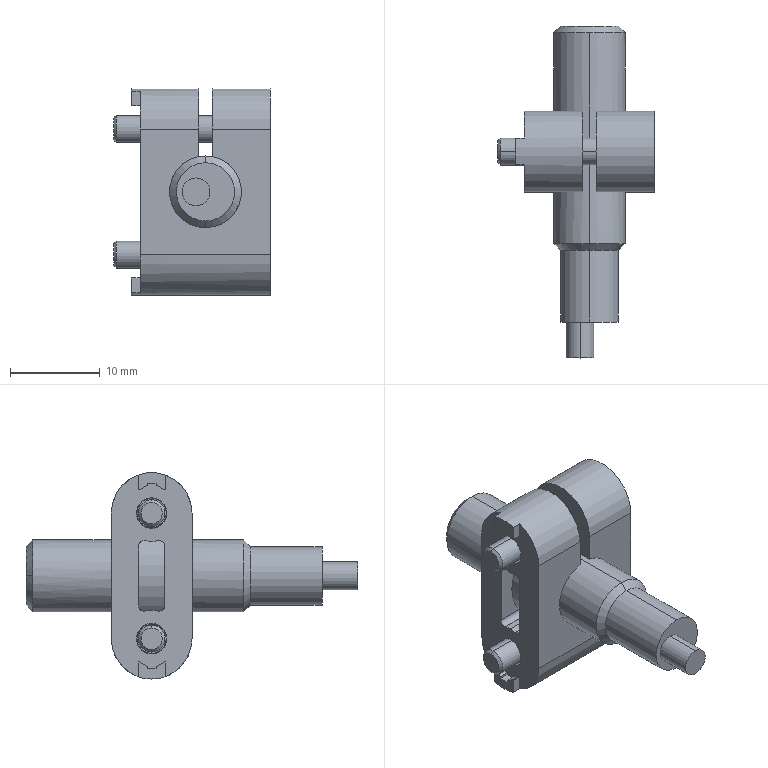Part | STEP file | _Sensor SBG - PAS42 B -1 | 1 solid | 124 faces | box 17.5 x 37 x 23 mm | volume 3611 mm3 | plane 56 | cylinder 44 | cone 20 | spline 4 | commonest cylinder face diameters 1 x6 1.2 x6 3 x4 3.4 x4 5.5 x4 9 x4